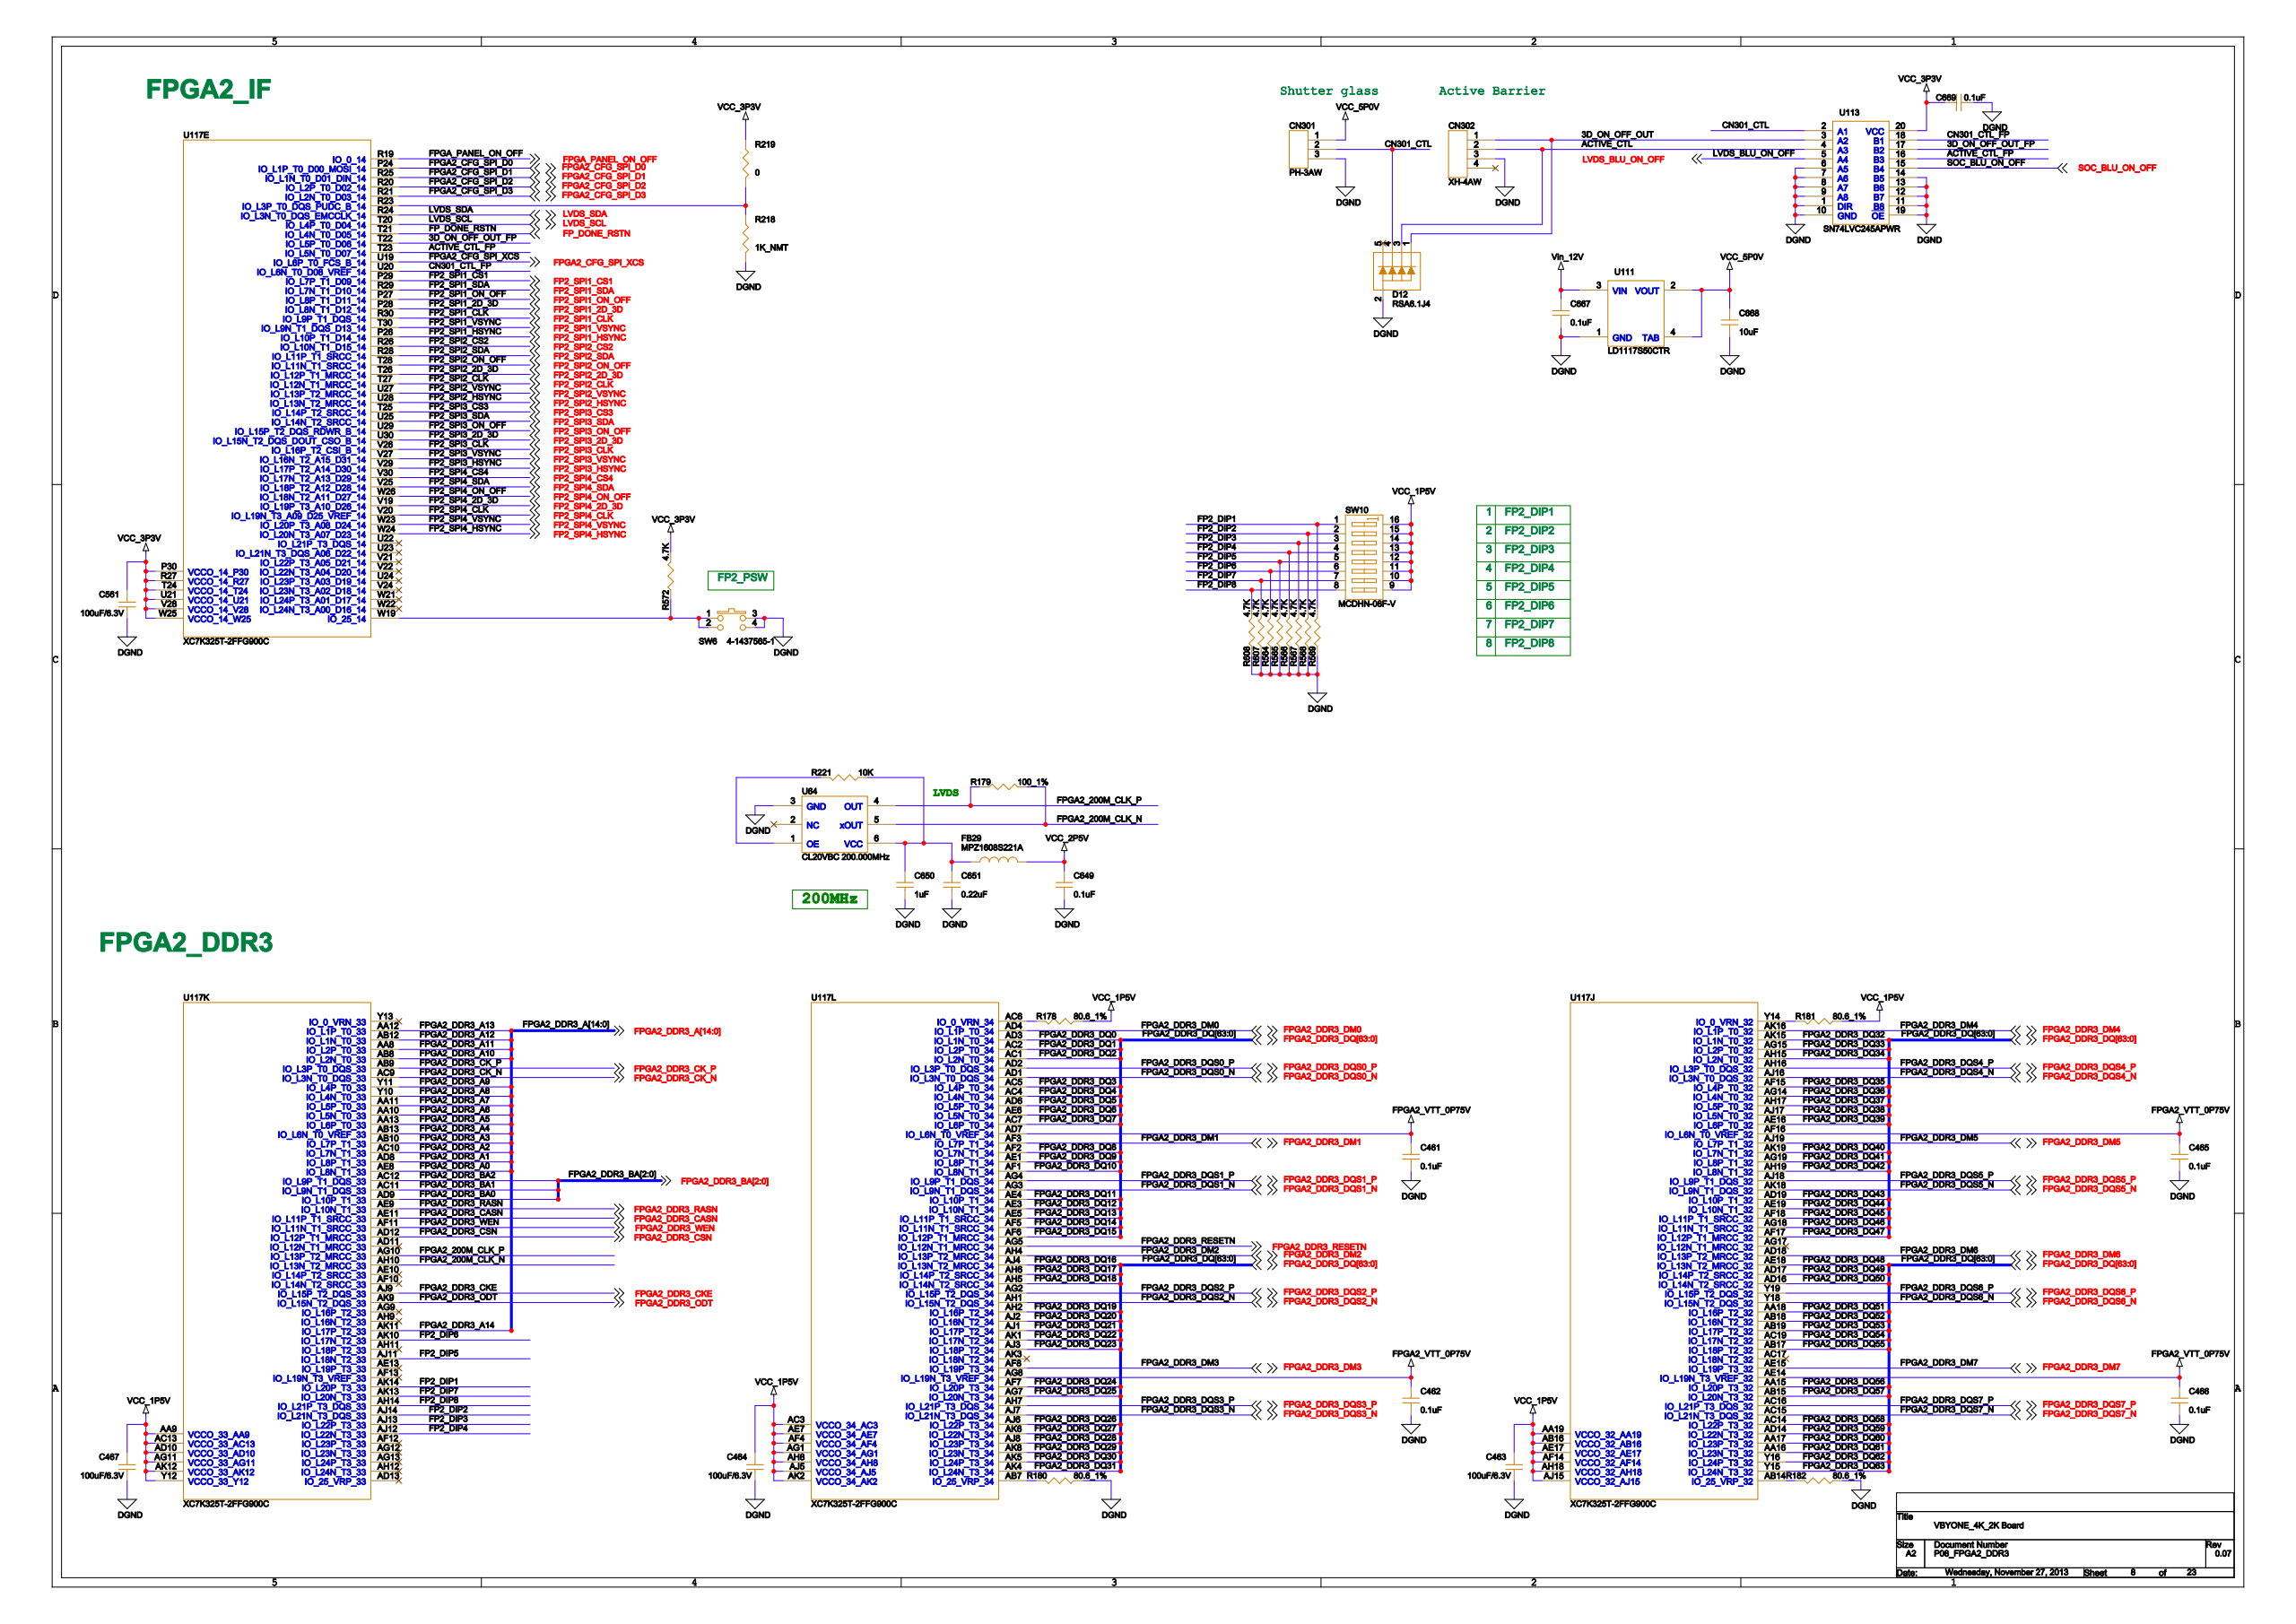Circuit board | Cadence Allegro | 1712 parts | 1495 nets | one sheet of the schematic
Parts on this sheet (reference | value | footprint):
C461 | 0.1uF | CRC1005RZAS
C462 | 0.1uF | CRC1005RZAS
C463 | 100uF/6.3V | CRC3225RZAS
C464 | 100uF/6.3V | CRC3225RZAS
C465 | 0.1uF | CRC1005RZAS
C466 | 0.1uF | CRC1005RZAS
C467 | 100uF/6.3V | CRC3225RZAS
C561 | 100uF/6.3V | CRC3225RZAS
C649 | 0.1uF | CRC1005RZAS
C650 | 1uF | CRC1608RZAS
C651 | 0.22uF | CRC1608RZAS
C667 | 0.1uF | CRC1005RZAS
C668 | 10uF | CRC2012RZAS
C669 | 0.1uF | CRC1005RZAS
CN301 | PH-3AW | CAD003LJAS
CN302 | XH-4AW | CAD004LKAS
D12 | RSA6.1J4 | DIC005RCAS
FB29 | MPZ1608S221A | LSC1608RZAS
R178 | 80.6_1% | CRC1608RZAS
R179 | 100_1% | CRC1005RZAS
R180 | 80.6_1% | CRC1608RZAS
R181 | 80.6_1% | CRC1608RZAS
R182 | 80.6_1% | CRC1608RZAS
R218 | 1K_NMT | CRC1608RZAS
R219 | 0 | CRC1608RZAS
R221 | 10K | CRC1005RZAS
R564 | 4.7K | CRC1005RZAS
R565 | 4.7K | CRC1005RZAS
R566 | 4.7K | CRC1005RZAS
R567 | 4.7K | CRC1005RZAS
R568 | 4.7K | CRC1005RZAS
R569 | 4.7K | CRC1005RZAS
R572 | 4.7K | CRC1005RZAS
R607 | 4.7K | CRC1005RZAS
R608 | 4.7K | CRC1005RZAS
SW6 | 4-1437565-1 | SWC004RZBS
SW10 | MCDHN-08F-V | SWC016RHBS
U20 | LMK03033CISQ | QFN048RCBS
U21 | K4B4G1646B-HCK0 | BGA096RFDS
U22 | K4B4G1646B-HCK0 | BGA096RFDS
U23 | K4B4G1646B-HCK0 | BGA096RFDS
U24 | K4B4G1646B-HCK0 | BGA096RFDS
U25 | K4B4G1646B-HCK0 | BGA096RFDS
U27 | K4B4G1646B-HCK0 | BGA096RFDS
U28 | K4B4G1646B-HCK0 | BGA096RFDS
U64 | CL20VBC 200.000MHz | XTC006RLDS
U111 | LD1117S50CTR | TRC004RZBS
U113 | SN74LVC245APWR | SOC020REAS
U117 | XC7K325T-2FFG900C | BGA900RGAS
Nets of these parts (net: part-pin ...):
VCC_3P3V: C561-2 C669-1 R219-1 R572-1 U113-20 U117-P30 U117-R27 U117-T24 U117-U21 U117-V28 U117-W25
DGND: C461-2 C462-2 C463-1 C464-1 C465-2 C466-2 C467-1 C561-1 C649-2 C650-2 C651-2 C667-2 C668-2 C669-2 CN301-3 CN302-3 D12-2 R180-1 R182-1 R218-2 R564-2 R565-2 R566-2 R567-2 R568-2 R569-2 R607-2 R608-2 SW6-3 SW6-4 U64-3 U111-1 U113-1 U113-6 U113-7 U113-8 U113-9 U113-10 U113-11 U113-12 U113-13 U113-14 U113-19 U20-1 U21-B1 U21-B3 U22-B1 U22-B3 U23-B1 U23-B3 U24-B1 U24-B3 U25-B1 U25-B3 U27-B1 U27-B3 U28-B1 U28-B3 U117-A1 U117-A2 U117-A5 U117-A6 U117-B4 U117-B8
VCC_1P5V: C463-2 C464-2 C467-2 R178-1 R181-1 SW10-9 SW10-10 SW10-11 SW10-12 SW10-13 SW10-14 SW10-15 SW10-16 U21-A1 U21-A8 U21-B2 U22-A1 U22-A8 U22-B2 U23-A1 U23-A8 U23-B2 U24-A1 U24-A8 U24-B2 U25-A1 U25-A8 U25-B2 U27-A1 U27-A8 U27-B2 U28-A1 U28-A8 U28-B2 U117-AA9 U117-AA19 U117-AB16 U117-AC3 U117-AC13 U117-AD10 U117-AE7 U117-AE17 U117-AF4 U117-AF14 U117-AG1 U117-AG11 U117-AH8 U117-AH18 U117-AJ5 U117-AJ15 U117-AK2 U117-AK12 U117-Y12
VIN_12V: C667-1 U111-3
FPGA2_VTT_0P75V: C461-1 C462-1 C465-1 C466-1 U117-AD7 U117-AE14 U117-AF16 U117-AG8
VCC_2P5V: C649-1 FB29-2
VCC_5P0V: C668-1 CN301-1 U111-2 U111-4
N19789227: C650-1 C651-1 FB29-1 R221-1 U64-6
LVDS_SDA: U117-R24
LVDS_SCL: U117-T20
SOC_BLU_ON_OFF: U113-15
CN301_CTL: CN301-2 D12-4 U113-2
3D_ON_OFF_OUT: CN302-1 D12-1 U113-3
ACTIVE_CTL: CN302-2 D12-3 U113-4
N16499579: R218-1 R219-2 U117-R23
FPGA2_200M_CLK_P: R179-1 U64-4 U117-AG10
FPGA2_200M_CLK_N: R179-2 U64-5 U117-AH10
FPGA_PANEL_ON_OFF: U117-R19
FPGA2_CFG_SPI_D0: U117-P24
FPGA2_CFG_SPI_D1: U117-R25
FPGA2_CFG_SPI_D2: U117-R20
FPGA2_CFG_SPI_D3: U117-R21
FP_DONE_RSTN: U117-T21
FP2_DIP6: R564-1 SW10-6 U117-AK10
FP2_DIP5: R565-1 SW10-5 U117-AJ11
FP2_DIP4: R566-1 SW10-4 U117-AJ12
FP2_DIP3: R567-1 SW10-3 U117-AJ13
FP2_DIP2: R568-1 SW10-2 U117-AJ14
FP2_DIP1: R569-1 SW10-1 U117-AK14
N19791494: R572-2 SW6-1 SW6-2 U117-W19
FP2_DIP7: R607-1 SW10-7 U117-AK13
FP2_DIP8: R608-1 SW10-8 U117-AH14
FPGA2_DDR3_CKE: U117-AJ9
FPGA2_DDR3_RESETN: U117-AG5
FPGA2_DDR3_ODT: U117-AK9
FPGA2_DDR3_CSN: U117-AD12
N19789221: R221-2 U64-1
FP2_SPI1_SDA: U117-R29
FP2_SPI1_CLK: U117-R30
FP2_SPI3_SDA: U117-U25
FP2_SPI3_CLK: U117-V26
FP2_SPI2_SDA: U117-R28
FP2_SPI2_CLK: U117-T27
FP2_SPI4_SDA: U117-V25
FP2_SPI4_CLK: U117-V20
FPGA2_DDR3_A0: U117-AE8
FPGA2_DDR3_A1: U117-AD8
FPGA2_DDR3_A2: U117-AC10
FPGA2_DDR3_A3: U117-AB10
FPGA2_DDR3_A4: U117-AB13
FPGA2_DDR3_A5: U117-AA13
FPGA2_DDR3_A6: U117-AA10
FPGA2_DDR3_A7: U117-AA11
FPGA2_DDR3_A8: U117-Y10
FPGA2_DDR3_A9: U117-Y11
FPGA2_DDR3_A10: U117-AB8
FPGA2_DDR3_A11: U117-AA8
FPGA2_DDR3_A12: U117-AB12
FPGA2_DDR3_A13: U117-AA12
FPGA2_DDR3_BA0: U117-AD9
FPGA2_DDR3_BA1: U117-AC11
FPGA2_DDR3_BA2: U117-AC12
FPGA2_DDR3_A14: U117-AK11
FPGA2_DDR3_RASN: U117-AE9
FPGA2_DDR3_CASN: U117-AE11
FPGA2_DDR3_WEN: U117-AF11
FPGA2_DDR3_CK_P: U117-AB9
FPGA2_DDR3_CK_N: U117-AC9
N17035091: R178-2 U117-AC6
N17034900: R180-2 U117-AB7
N18039823: R181-2 U117-Y14
N18039228: R182-2 U117-AB14
FPGA2_CFG_SPI_XCS: U117-U19
FP2_SPI1_ON_OFF: U117-P27
FP2_SPI2_ON_OFF: U117-T28
FP2_SPI3_ON_OFF: U117-U29
FP2_SPI4_ON_OFF: U117-W26
CN301_CTL_FP: U113-18 U117-U20
3D_ON_OFF_OUT_FP: U113-17 U117-T22
LVDS_BLU_ON_OFF: U113-5
ACTIVE_CTL_FP: U113-16 U117-T23
FP2_SPI1_HSYNC: U117-P26
FP2_SPI1_VSYNC: U117-T30
FP2_SPI1_CS1: U117-P29
FP2_SPI1_2D_3D: U117-P28
FP2_SPI2_HSYNC: U117-U28
FP2_SPI2_VSYNC: U117-U27
FP2_SPI2_CS2: U117-R26
FP2_SPI2_2D_3D: U117-T26
FP2_SPI3_HSYNC: U117-V29
FP2_SPI3_VSYNC: U117-V27
FP2_SPI3_CS3: U117-T25
FP2_SPI3_2D_3D: U117-U30
FP2_SPI4_HSYNC: U117-W24
FP2_SPI4_VSYNC: U117-W23
FP2_SPI4_CS4: U117-V30
FP2_SPI4_2D_3D: U117-V19
FPGA2_DDR3_DQ22: U117-AK1
FPGA2_DDR3_DQ21: U117-AJ1
FPGA2_DDR3_DQS2_N: U117-AH1
FPGA2_DDR3_DQ10: U117-AF1
FPGA2_DDR3_DQ9: U117-AE1
FPGA2_DDR3_DQS0_N: U117-AD1
FPGA2_DDR3_DQ2: U117-AC1
FPGA2_DDR3_DQ20: U117-AJ2
FPGA2_DDR3_DQ19: U117-AH2
FPGA2_DDR3_DQS2_P: U117-AG2
FPGA2_DDR3_DQ8: U117-AF2
FPGA2_DDR3_DQS0_P: U117-AD2
FPGA2_DDR3_DQ1: U117-AC2
FPGA2_DDR3_DQ23: U117-AJ3
FPGA2_DDR3_DQS1_N: U25-B7 U117-AG3
FPGA2_DDR3_DM1: U117-AF3
FPGA2_DDR3_DQ12: U25-A7 U117-AE3
FPGA2_DDR3_DQ0: U117-AD3
FPGA2_DDR3_DQ31: U117-AK4
FPGA2_DDR3_DQ16: U117-AJ4
FPGA2_DDR3_DM2: U117-AH4
FPGA2_DDR3_DQS1_P: U117-AG4
FPGA2_DDR3_DQ11: U117-AE4
FPGA2_DDR3_DM0: U117-AD4
FPGA2_DDR3_DQ4: U117-AC4
FPGA2_DDR3_DQ30: U117-AK5
FPGA2_DDR3_DQ18: U117-AH5
FPGA2_DDR3_DQ14: U25-B8 U117-AF5
FPGA2_DDR3_DQ13: U25-A2 U117-AE5
FPGA2_DDR3_DQ3: U117-AC5
FPGA2_DDR3_DQ27: U117-AK6
FPGA2_DDR3_DQ26: U117-AJ6
FPGA2_DDR3_DQ17: U117-AH6
FPGA2_DDR3_DQ15: U25-A3 U117-AF6
FPGA2_DDR3_DQ6: U117-AE6
FPGA2_DDR3_DQ5: U117-AD6
FPGA2_DDR3_DQS3_N: U117-AJ7
FPGA2_DDR3_DQS3_P: U117-AH7
FPGA2_DDR3_DQ25: U117-AG7
FPGA2_DDR3_DQ24: U117-AF7
FPGA2_DDR3_DQ7: U117-AC7
FPGA2_DDR3_DQ29: U117-AK8
FPGA2_DDR3_DQ28: U117-AJ8
FPGA2_DDR3_DM3: U117-AF8
FPGA2_DDR3_DQ36: U117-AG14
FPGA2_DDR3_DQ59: U117-AD14
FPGA2_DDR3_DQ58: U117-AC14
FPGA2_DDR3_DQ32: U117-AK15
FPGA2_DDR3_DQ34: U117-AH15
FPGA2_DDR3_DQ33: U117-AG15
FPGA2_DDR3_DQ35: U117-AF15
FPGA2_DDR3_DM7: U117-AE15
FPGA2_DDR3_DQS7_N: U28-B7 U117-AC15
FPGA2_DDR3_DQ57: U117-AB15
FPGA2_DDR3_DQ56: U117-AA15
FPGA2_DDR3_DQ63: U28-A3 U117-Y15
FPGA2_DDR3_DM4: U117-AK16
FPGA2_DDR3_DQS4_N: U117-AJ16
FPGA2_DDR3_DQS4_P: U117-AH16
FPGA2_DDR3_DQ39: U117-AE16
FPGA2_DDR3_DQ50: U117-AD16
FPGA2_DDR3_DQS7_P: U117-AC16
FPGA2_DDR3_DQ61: U28-A2 U117-AA16
FPGA2_DDR3_DQ62: U28-B8 U117-Y16
FPGA2_DDR3_DQ38: U117-AJ17
FPGA2_DDR3_DQ37: U117-AH17
FPGA2_DDR3_DQ47: U27-A3 U117-AF17
FPGA2_DDR3_DQ49: U117-AD17
FPGA2_DDR3_DQ55: U117-AB17
FPGA2_DDR3_DQ60: U28-A7 U117-AA17
FPGA2_DDR3_DQS5_N: U27-B7 U117-AK18
FPGA2_DDR3_DQS5_P: U117-AJ18
FPGA2_DDR3_DQ46: U27-B8 U117-AG18
FPGA2_DDR3_DQ45: U27-A2 U117-AF18
FPGA2_DDR3_DQ48: U117-AE18
FPGA2_DDR3_DM6: U117-AD18
FPGA2_DDR3_DQ52: U117-AB18
FPGA2_DDR3_DQ51: U117-AA18
FPGA2_DDR3_DQS6_N: U117-Y18
FPGA2_DDR3_DQ40: U117-AK19
FPGA2_DDR3_DM5: U117-AJ19
FPGA2_DDR3_DQ42: U117-AH19
FPGA2_DDR3_DQ41: U117-AG19
FPGA2_DDR3_DQ44: U27-A7 U117-AE19
FPGA2_DDR3_DQ43: U117-AD19
FPGA2_DDR3_DQ54: U117-AC19
FPGA2_DDR3_DQ53: U117-AB19
FPGA2_DDR3_DQS6_P: U117-Y19